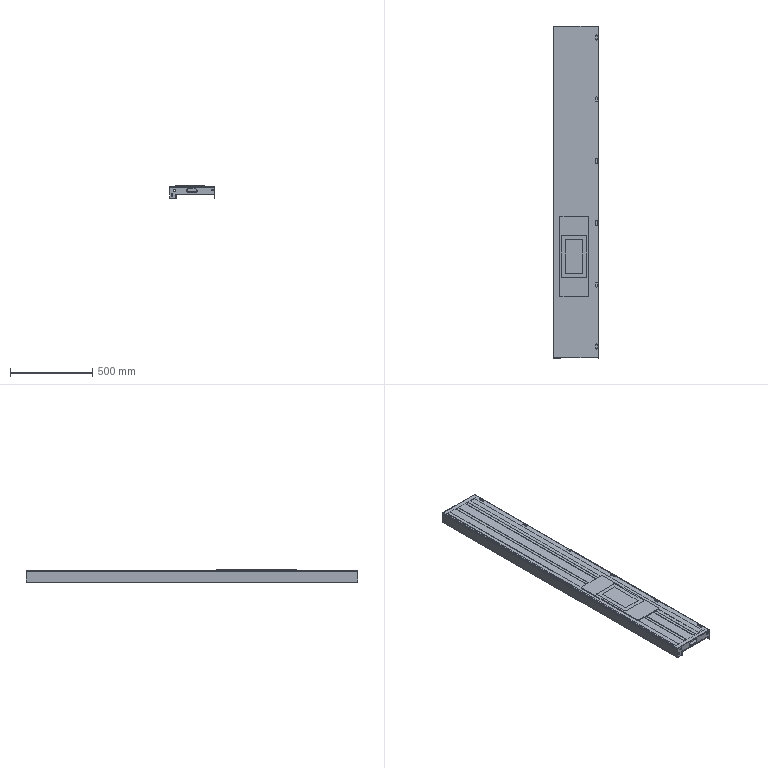Part | 14 solids | 787 faces | box 276 x 2016 x 79 mm | volume 6761459 mm3 | plane 494 | cylinder 293 | commonest cylinder face diameters 8 x60 6 x56 6.2 x28 2 x20 9 x18 3.6 x12